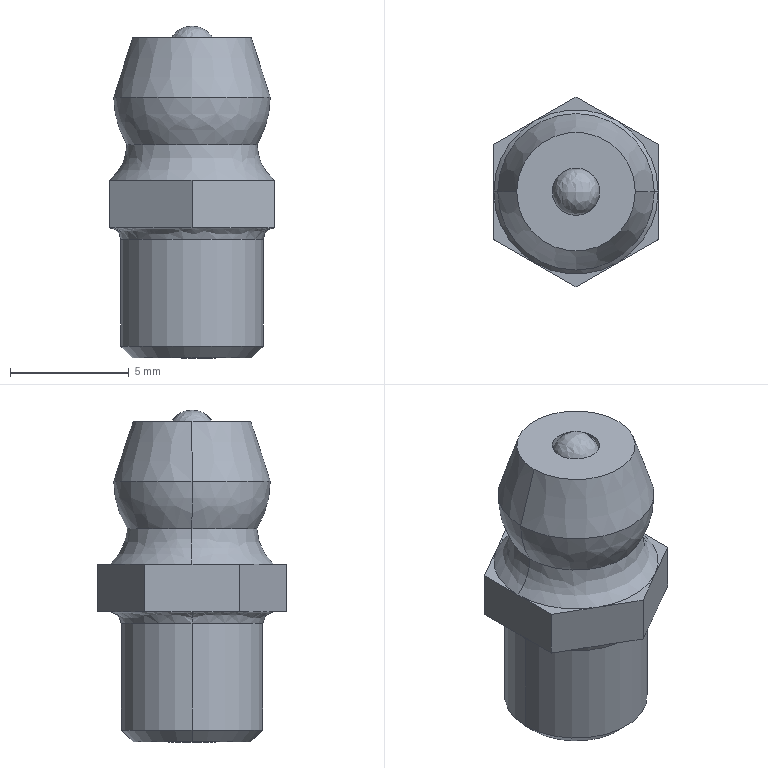Part | STEP file | M6 grease nipple^FTH120-PD-direct-drive motor | 2 solids | 36 faces | box 6.928 x 8 x 13.96 mm | volume 368.725 mm3 | plane 20 | spline 8 | cylinder 4 | cone 4 | commonest cylinder face diameters 2 x2 6 x2
STEP:
#1=CARTESIAN_POINT('',(-1.,0.,13.));
#2=VERTEX_POINT('',#1);
#3=CARTESIAN_POINT('',(1.,0.,13.));
#4=VERTEX_POINT('',#3);
#5=CARTESIAN_POINT('',(0.,0.,13.));
#6=DIRECTION('',(0.,0.,-1.));
#7=DIRECTION('',(-1.,0.,0.));
#8=AXIS2_PLACEMENT_3D('',#5,#6,#7);
#9=CIRCLE('',#8,1.);
#10=EDGE_CURVE('',#2,#4,#9,.T.);
#11=ORIENTED_EDGE('',*,*,#10,.F.);
#12=CARTESIAN_POINT('',(0.,0.,13.));
#13=DIRECTION('',(0.,0.,1.));
#14=DIRECTION('',(-1.,0.,0.));
#15=AXIS2_PLACEMENT_3D('',#12,#13,#14);
#16=CIRCLE('',#15,1.);
#17=EDGE_CURVE('',#2,#4,#16,.T.);
#18=ORIENTED_EDGE('',*,*,#17,.T.);
#19=EDGE_LOOP('',(#11,#18));
#20=FACE_OUTER_BOUND('',#19,.T.);
#21=CARTESIAN_POINT('',(-1.,0.,13.));
#22=CARTESIAN_POINT('',(-1.,0.,13.));
#23=CARTESIAN_POINT('',(-1.,0.,13.));
#24=CARTESIAN_POINT('',(-1.,0.,13.));
#25=CARTESIAN_POINT('',(-1.,-2.,13.));
#26=CARTESIAN_POINT('',(-1.,-2.,17.));
#27=CARTESIAN_POINT('',(-1.,2.,17.));
#28=CARTESIAN_POINT('',(-1.,2.,13.));
#29=CARTESIAN_POINT('',(1.,-2.,13.));
#30=CARTESIAN_POINT('',(1.,-2.,17.));
#31=CARTESIAN_POINT('',(1.,2.,17.));
#32=CARTESIAN_POINT('',(1.,2.,13.));
#33=CARTESIAN_POINT('',(1.,0.,13.));
#34=CARTESIAN_POINT('',(1.,0.,13.));
#35=CARTESIAN_POINT('',(1.,0.,13.));
#36=CARTESIAN_POINT('',(1.,0.,13.));
#37=(BOUNDED_SURFACE()B_SPLINE_SURFACE(3,3,((#21,#22,#23,#24),(#25,#26,#27,#28),(#29,#30,#31,#32),(#33,#34,#35,#36)),.UNSPECIFIED.,.F.,.F.,.T.)B_SPLINE_SURFACE_WITH_KNOTS((4,4),(4,4),(0.,1.),(0.,1.),.UNSPECIFIED.)GEOMETRIC_REPRESENTATION_ITEM()RATIONAL_B_SPLINE_SURFACE(((1.,0.3333,0.3333,1.),(0.3333,0.1111,0.1111,0.3333),(0.3333,0.1111,0.1111,0.3333),(1.,0.3333,0.3333,1.)))REPRESENTATION_ITEM('')SURFACE());
#38=ADVANCED_FACE('',(#20),#37,.T.);
#39=ORIENTED_EDGE('',*,*,#17,.F.);
#40=ORIENTED_EDGE('',*,*,#10,.T.);
#41=EDGE_LOOP('',(#39,#40));
#42=FACE_OUTER_BOUND('',#41,.T.);
#43=CARTESIAN_POINT('',(-1.,0.,13.));
#44=CARTESIAN_POINT('',(-1.,0.,13.));
#45=CARTESIAN_POINT('',(-1.,0.,13.));
#46=CARTESIAN_POINT('',(-1.,0.,13.));
#47=CARTESIAN_POINT('',(-1.,2.,13.));
#48=CARTESIAN_POINT('',(-1.,2.,9.));
#49=CARTESIAN_POINT('',(-1.,-2.,9.));
#50=CARTESIAN_POINT('',(-1.,-2.,13.));
#51=CARTESIAN_POINT('',(1.,2.,13.));
#52=CARTESIAN_POINT('',(1.,2.,9.));
#53=CARTESIAN_POINT('',(1.,-2.,9.));
#54=CARTESIAN_POINT('',(1.,-2.,13.));
#55=CARTESIAN_POINT('',(1.,0.,13.));
#56=CARTESIAN_POINT('',(1.,0.,13.));
#57=CARTESIAN_POINT('',(1.,0.,13.));
#58=CARTESIAN_POINT('',(1.,0.,13.));
#59=(BOUNDED_SURFACE()B_SPLINE_SURFACE(3,3,((#43,#44,#45,#46),(#47,#48,#49,#50),(#51,#52,#53,#54),(#55,#56,#57,#58)),.UNSPECIFIED.,.F.,.F.,.T.)B_SPLINE_SURFACE_WITH_KNOTS((4,4),(4,4),(0.,1.),(0.,1.),.UNSPECIFIED.)GEOMETRIC_REPRESENTATION_ITEM()RATIONAL_B_SPLINE_SURFACE(((1.,0.3333,0.3333,1.),(0.3333,0.1111,0.1111,0.3333),(0.3333,0.1111,0.1111,0.3333),(1.,0.3333,0.3333,1.)))REPRESENTATION_ITEM('')SURFACE());
#60=ADVANCED_FACE('',(#42),#59,.T.);
#61=CLOSED_SHELL('',(#38,#60));
#62=MANIFOLD_SOLID_BREP('',#61);
#63=CARTESIAN_POINT('',(3.464,0.,5.499));
#64=VERTEX_POINT('',#63);
#65=CARTESIAN_POINT('',(3.464,0.5,5.5));
#66=VERTEX_POINT('',#65);
#67=CARTESIAN_POINT('',(3.464,0.,5.499));
#68=CARTESIAN_POINT('',(3.464,0.1667,5.499));
#69=CARTESIAN_POINT('',(3.464,0.3333,5.5));
#70=CARTESIAN_POINT('',(3.464,0.5,5.5));
#71=B_SPLINE_CURVE_WITH_KNOTS('',3,(#67,#68,#69,#70),.UNSPECIFIED.,.F.,.F.,(4,4),(0.,0.0005),.UNSPECIFIED.);
#72=EDGE_CURVE('',#64,#66,#71,.T.);
#73=ORIENTED_EDGE('',*,*,#72,.F.);
#74=CARTESIAN_POINT('',(3.,0.,5.));
#75=VERTEX_POINT('',#74);
#76=CARTESIAN_POINT('',(3.5,0.,5.));
#77=DIRECTION('',(0.,-1.,0.));
#78=DIRECTION('',(1.,0.,0.));
#79=AXIS2_PLACEMENT_3D('',#76,#77,#78);
#80=CIRCLE('',#79,0.5);
#81=EDGE_CURVE('',#64,#75,#80,.T.);
#82=ORIENTED_EDGE('',*,*,#81,.T.);
#83=CARTESIAN_POINT('',(-3.,0.,5.));
#84=VERTEX_POINT('',#83);
#85=CARTESIAN_POINT('',(0.,0.,5.));
#86=DIRECTION('',(0.,0.,-1.));
#87=DIRECTION('',(-1.,0.,0.));
#88=AXIS2_PLACEMENT_3D('',#85,#86,#87);
#89=CIRCLE('',#88,3.);
#90=EDGE_CURVE('',#84,#75,#89,.T.);
#91=ORIENTED_EDGE('',*,*,#90,.F.);
#92=CARTESIAN_POINT('',(-3.464,0.,5.499));
#93=VERTEX_POINT('',#92);
#94=CARTESIAN_POINT('',(-3.5,0.,5.));
#95=DIRECTION('',(0.,1.,0.));
#96=DIRECTION('',(-1.,0.,0.));
#97=AXIS2_PLACEMENT_3D('',#94,#95,#96);
#98=CIRCLE('',#97,0.5);
#99=EDGE_CURVE('',#93,#84,#98,.T.);
#100=ORIENTED_EDGE('',*,*,#99,.F.);
#101=CARTESIAN_POINT('',(-3.464,0.5,5.5));
#102=VERTEX_POINT('',#101);
#103=CARTESIAN_POINT('',(-3.464,0.5,5.5));
#104=CARTESIAN_POINT('',(-3.464,0.3333,5.5));
#105=CARTESIAN_POINT('',(-3.464,0.1667,5.499));
#106=CARTESIAN_POINT('',(-3.464,0.,5.499));
#107=B_SPLINE_CURVE_WITH_KNOTS('',3,(#103,#104,#105,#106),.UNSPECIFIED.,.F.,.F.,(4,4),(-0.0005,0.),.UNSPECIFIED.);
#108=EDGE_CURVE('',#102,#93,#107,.T.);
#109=ORIENTED_EDGE('',*,*,#108,.F.);
#110=CARTESIAN_POINT('',(-2.165,2.75,5.5));
#111=VERTEX_POINT('',#110);
#112=CARTESIAN_POINT('',(-2.165,2.75,5.5));
#113=CARTESIAN_POINT('',(-2.518,2.472,5.5));
#114=CARTESIAN_POINT('',(-2.807,2.139,5.5));
#115=CARTESIAN_POINT('',(-3.256,1.361,5.5));
#116=CARTESIAN_POINT('',(-3.4,0.9446,5.5));
#117=CARTESIAN_POINT('',(-3.464,0.5,5.5));
#118=B_SPLINE_CURVE_WITH_KNOTS('',3,(#112,#113,#114,#115,#116,#117),.UNSPECIFIED.,.F.,.F.,(4,2,4),(0.,0.5,1.),.UNSPECIFIED.);
#119=EDGE_CURVE('',#111,#102,#118,.T.);
#120=ORIENTED_EDGE('',*,*,#119,.F.);
#121=CARTESIAN_POINT('',(-1.299,3.25,5.5));
#122=VERTEX_POINT('',#121);
#123=CARTESIAN_POINT('',(-1.299,3.25,5.5));
#124=CARTESIAN_POINT('',(-1.443,3.167,5.5));
#125=CARTESIAN_POINT('',(-1.588,3.083,5.499));
#126=CARTESIAN_POINT('',(-1.732,3.,5.499));
#127=CARTESIAN_POINT('',(-1.876,2.917,5.499));
#128=CARTESIAN_POINT('',(-2.021,2.833,5.5));
#129=CARTESIAN_POINT('',(-2.165,2.75,5.5));
#130=B_SPLINE_CURVE_WITH_KNOTS('',3,(#123,#124,#125,#126,#127,#128,#129),.UNSPECIFIED.,.F.,.F.,(4,3,4),(0.,0.0005,0.001),.UNSPECIFIED.);
#131=EDGE_CURVE('',#122,#111,#130,.T.);
#132=ORIENTED_EDGE('',*,*,#131,.F.);
#133=CARTESIAN_POINT('',(1.299,3.25,5.5));
#134=VERTEX_POINT('',#133);
#135=CARTESIAN_POINT('',(1.299,3.25,5.5));
#136=CARTESIAN_POINT('',(0.8822,3.417,5.5));
#137=CARTESIAN_POINT('',(0.4489,3.5,5.5));
#138=CARTESIAN_POINT('',(-0.4489,3.5,5.5));
#139=CARTESIAN_POINT('',(-0.8819,3.417,5.5));
#140=CARTESIAN_POINT('',(-1.299,3.25,5.5));
#141=B_SPLINE_CURVE_WITH_KNOTS('',3,(#135,#136,#137,#138,#139,#140),.UNSPECIFIED.,.F.,.F.,(4,2,4),(0.,0.5,1.),.UNSPECIFIED.);
#142=EDGE_CURVE('',#134,#122,#141,.T.);
#143=ORIENTED_EDGE('',*,*,#142,.F.);
#144=CARTESIAN_POINT('',(2.165,2.75,5.5));
#145=VERTEX_POINT('',#144);
#146=CARTESIAN_POINT('',(2.165,2.75,5.5));
#147=CARTESIAN_POINT('',(2.021,2.833,5.5));
#148=CARTESIAN_POINT('',(1.876,2.917,5.499));
#149=CARTESIAN_POINT('',(1.732,3.,5.499));
#150=CARTESIAN_POINT('',(1.588,3.083,5.499));
#151=CARTESIAN_POINT('',(1.443,3.167,5.5));
#152=CARTESIAN_POINT('',(1.299,3.25,5.5));
#153=B_SPLINE_CURVE_WITH_KNOTS('',3,(#146,#147,#148,#149,#150,#151,#152),.UNSPECIFIED.,.F.,.F.,(4,3,4),(0.,0.0005,0.001),.UNSPECIFIED.);
#154=EDGE_CURVE('',#145,#134,#153,.T.);
#155=ORIENTED_EDGE('',*,*,#154,.F.);
#156=CARTESIAN_POINT('',(3.464,0.5,5.5));
#157=CARTESIAN_POINT('',(3.4,0.9443,5.5));
#158=CARTESIAN_POINT('',(3.255,1.361,5.5));
#159=CARTESIAN_POINT('',(2.807,2.139,5.5));
#160=CARTESIAN_POINT('',(2.518,2.472,5.5));
#161=CARTESIAN_POINT('',(2.165,2.75,5.5));
#162=B_SPLINE_CURVE_WITH_KNOTS('',3,(#156,#157,#158,#159,#160,#161),.UNSPECIFIED.,.F.,.F.,(4,2,4),(0.,0.5,1.),.UNSPECIFIED.);
#163=EDGE_CURVE('',#66,#145,#162,.T.);
#164=ORIENTED_EDGE('',*,*,#163,.F.);
#165=EDGE_LOOP('',(#73,#82,#91,#100,#109,#120,#132,#143,#155,#164));
#166=FACE_OUTER_BOUND('',#165,.T.);
#167=CARTESIAN_POINT('',(-3.5,0.,5.5));
#168=CARTESIAN_POINT('',(-3.5,7.,5.5));
#169=CARTESIAN_POINT('',(3.5,7.,5.5));
#170=CARTESIAN_POINT('',(3.5,0.,5.5));
#171=CARTESIAN_POINT('',(-3.207,0.,5.5));
#172=CARTESIAN_POINT('',(-3.207,6.414,5.5));
#173=CARTESIAN_POINT('',(3.207,6.414,5.5));
#174=CARTESIAN_POINT('',(3.207,0.,5.5));
#175=CARTESIAN_POINT('',(-3.,0.,5.293));
#176=CARTESIAN_POINT('',(-3.,6.,5.293));
#177=CARTESIAN_POINT('',(3.,6.,5.293));
#178=CARTESIAN_POINT('',(3.,0.,5.293));
#179=CARTESIAN_POINT('',(-3.,0.,5.));
#180=CARTESIAN_POINT('',(-3.,6.,5.));
#181=CARTESIAN_POINT('',(3.,6.,5.));
#182=CARTESIAN_POINT('',(3.,0.,5.));
#183=(BOUNDED_SURFACE()B_SPLINE_SURFACE(3,3,((#167,#168,#169,#170),(#171,#172,#173,#174),(#175,#176,#177,#178),(#179,#180,#181,#182)),.UNSPECIFIED.,.F.,.F.,.T.)B_SPLINE_SURFACE_WITH_KNOTS((4,4),(4,4),(0.,1.),(0.,1.),.UNSPECIFIED.)GEOMETRIC_REPRESENTATION_ITEM()RATIONAL_B_SPLINE_SURFACE(((1.,0.3333,0.3333,1.),(0.8047,0.2682,0.2682,0.8047),(0.8047,0.2682,0.2682,0.8047),(1.,0.3333,0.3333,1.)))REPRESENTATION_ITEM('')SURFACE());
#184=ADVANCED_FACE('',(#166),#183,.F.);
#185=CARTESIAN_POINT('',(2.75,0.,9.));
#186=VERTEX_POINT('',#185);
#187=CARTESIAN_POINT('',(-2.75,0.,9.));
#188=VERTEX_POINT('',#187);
#189=CARTESIAN_POINT('',(0.,0.,9.));
#190=DIRECTION('',(0.,0.,1.));
#191=DIRECTION('',(-1.,0.,0.));
#192=AXIS2_PLACEMENT_3D('',#189,#190,#191);
#193=CIRCLE('',#192,2.75);
#194=EDGE_CURVE('',#186,#188,#193,.T.);
#195=ORIENTED_EDGE('',*,*,#194,.F.);
#196=CARTESIAN_POINT('',(3.464,0.,7.5));
#197=VERTEX_POINT('',#196);
#198=CARTESIAN_POINT('',(4.682,0.,9.));
#199=DIRECTION('',(0.,-1.,0.));
#200=DIRECTION('',(1.,0.,0.));
#201=AXIS2_PLACEMENT_3D('',#198,#199,#200);
#202=CIRCLE('',#201,1.932);
#203=EDGE_CURVE('',#186,#197,#202,.T.);
#204=ORIENTED_EDGE('',*,*,#203,.T.);
#205=CARTESIAN_POINT('',(1.732,3.,7.5));
#206=VERTEX_POINT('',#205);
#207=CARTESIAN_POINT('',(0.,0.,7.5));
#208=DIRECTION('',(0.,0.,-1.));
#209=DIRECTION('',(-1.,0.,0.));
#210=AXIS2_PLACEMENT_3D('',#207,#208,#209);
#211=CIRCLE('',#210,3.464);
#212=EDGE_CURVE('',#206,#197,#211,.T.);
#213=ORIENTED_EDGE('',*,*,#212,.F.);
#214=CARTESIAN_POINT('',(-1.732,3.,7.5));
#215=VERTEX_POINT('',#214);
#216=CARTESIAN_POINT('',(0.,0.,7.5));
#217=DIRECTION('',(0.,0.,-1.));
#218=DIRECTION('',(-1.,0.,0.));
#219=AXIS2_PLACEMENT_3D('',#216,#217,#218);
#220=CIRCLE('',#219,3.464);
#221=EDGE_CURVE('',#215,#206,#220,.T.);
#222=ORIENTED_EDGE('',*,*,#221,.F.);
#223=CARTESIAN_POINT('',(-3.464,0.,7.5));
#224=VERTEX_POINT('',#223);
#225=CARTESIAN_POINT('',(0.,0.,7.5));
#226=DIRECTION('',(0.,0.,-1.));
#227=DIRECTION('',(-1.,0.,0.));
#228=AXIS2_PLACEMENT_3D('',#225,#226,#227);
#229=CIRCLE('',#228,3.464);
#230=EDGE_CURVE('',#224,#215,#229,.T.);
#231=ORIENTED_EDGE('',*,*,#230,.F.);
#232=CARTESIAN_POINT('',(-4.682,0.,9.));
#233=DIRECTION('',(0.,1.,0.));
#234=DIRECTION('',(-1.,0.,0.));
#235=AXIS2_PLACEMENT_3D('',#232,#233,#234);
#236=CIRCLE('',#235,1.932);
#237=EDGE_CURVE('',#188,#224,#236,.T.);
#238=ORIENTED_EDGE('',*,*,#237,.F.);
#239=EDGE_LOOP('',(#195,#204,#213,#222,#231,#238));
#240=FACE_OUTER_BOUND('',#239,.T.);
#241=CARTESIAN_POINT('',(-2.75,0.,9.));
#242=CARTESIAN_POINT('',(-2.75,5.5,9.));
#243=CARTESIAN_POINT('',(2.75,5.5,9.));
#244=CARTESIAN_POINT('',(2.75,0.,9.));
#245=CARTESIAN_POINT('',(-2.75,0.,8.408));
#246=CARTESIAN_POINT('',(-2.75,5.5,8.408));
#247=CARTESIAN_POINT('',(2.75,5.5,8.408));
#248=CARTESIAN_POINT('',(2.75,0.,8.408));
#249=CARTESIAN_POINT('',(-3.005,0.,7.873));
#250=CARTESIAN_POINT('',(-3.005,6.009,7.873));
#251=CARTESIAN_POINT('',(3.005,6.009,7.873));
#252=CARTESIAN_POINT('',(3.005,0.,7.873));
#253=CARTESIAN_POINT('',(-3.464,0.,7.5));
#254=CARTESIAN_POINT('',(-3.464,6.928,7.5));
#255=CARTESIAN_POINT('',(3.464,6.928,7.5));
#256=CARTESIAN_POINT('',(3.464,0.,7.5));
#257=(BOUNDED_SURFACE()B_SPLINE_SURFACE(3,3,((#241,#242,#243,#244),(#245,#246,#247,#248),(#249,#250,#251,#252),(#253,#254,#255,#256)),.UNSPECIFIED.,.F.,.F.,.T.)B_SPLINE_SURFACE_WITH_KNOTS((4,4),(4,4),(0.,1.),(0.,1.),.UNSPECIFIED.)GEOMETRIC_REPRESENTATION_ITEM()RATIONAL_B_SPLINE_SURFACE(((1.,0.3333,0.3333,1.),(0.9353,0.3118,0.3118,0.9353),(0.9353,0.3118,0.3118,0.9353),(1.,0.3333,0.3333,1.)))REPRESENTATION_ITEM('')SURFACE());
#258=ADVANCED_FACE('',(#240),#257,.F.);
#259=CARTESIAN_POINT('',(0.,0.,9.));
#260=DIRECTION('',(0.,0.,1.));
#261=DIRECTION('',(-1.,0.,0.));
#262=AXIS2_PLACEMENT_3D('',#259,#260,#261);
#263=CIRCLE('',#262,2.75);
#264=EDGE_CURVE('',#188,#186,#263,.T.);
#265=ORIENTED_EDGE('',*,*,#264,.T.);
#266=CARTESIAN_POINT('',(3.3,0.,11.));
#267=VERTEX_POINT('',#266);
#268=CARTESIAN_POINT('',(-0.6999,0.,11.024));
#269=DIRECTION('',(0.,-1.,0.));
#270=DIRECTION('',(1.,0.,0.));
#271=AXIS2_PLACEMENT_3D('',#268,#269,#270);
#272=CIRCLE('',#271,4.);
#273=EDGE_CURVE('',#186,#267,#272,.T.);
#274=ORIENTED_EDGE('',*,*,#273,.T.);
#275=CARTESIAN_POINT('',(-3.3,0.,11.));
#276=VERTEX_POINT('',#275);
#277=CARTESIAN_POINT('',(0.,0.,11.));
#278=DIRECTION('',(0.,0.,1.));
#279=DIRECTION('',(-1.,0.,0.));
#280=AXIS2_PLACEMENT_3D('',#277,#278,#279);
#281=CIRCLE('',#280,3.3);
#282=EDGE_CURVE('',#276,#267,#281,.T.);
#283=ORIENTED_EDGE('',*,*,#282,.F.);
#284=CARTESIAN_POINT('',(0.6999,0.,11.024));
#285=DIRECTION('',(0.,1.,0.));
#286=DIRECTION('',(-1.,0.,0.));
#287=AXIS2_PLACEMENT_3D('',#284,#285,#286);
#288=CIRCLE('',#287,4.);
#289=EDGE_CURVE('',#188,#276,#288,.T.);
#290=ORIENTED_EDGE('',*,*,#289,.F.);
#291=EDGE_LOOP('',(#265,#274,#283,#290));
#292=FACE_OUTER_BOUND('',#291,.T.);
#293=CARTESIAN_POINT('',(2.75,0.,9.));
#294=CARTESIAN_POINT('',(2.75,-5.5,9.));
#295=CARTESIAN_POINT('',(-2.75,-5.5,9.));
#296=CARTESIAN_POINT('',(-2.75,0.,9.));
#297=CARTESIAN_POINT('',(3.108,0.,9.61));
#298=CARTESIAN_POINT('',(3.108,-6.216,9.61));
#299=CARTESIAN_POINT('',(-3.108,-6.216,9.61));
#300=CARTESIAN_POINT('',(-3.108,0.,9.61));
#301=CARTESIAN_POINT('',(3.296,0.,10.292));
#302=CARTESIAN_POINT('',(3.296,-6.591,10.292));
#303=CARTESIAN_POINT('',(-3.296,-6.591,10.292));
#304=CARTESIAN_POINT('',(-3.296,0.,10.292));
#305=CARTESIAN_POINT('',(3.3,0.,11.));
#306=CARTESIAN_POINT('',(3.3,-6.6,11.));
#307=CARTESIAN_POINT('',(-3.3,-6.6,11.));
#308=CARTESIAN_POINT('',(-3.3,0.,11.));
#309=(BOUNDED_SURFACE()B_SPLINE_SURFACE(3,3,((#293,#294,#295,#296),(#297,#298,#299,#300),(#301,#302,#303,#304),(#305,#306,#307,#308)),.UNSPECIFIED.,.F.,.F.,.T.)B_SPLINE_SURFACE_WITH_KNOTS((4,4),(4,4),(0.,1.),(0.,1.),.UNSPECIFIED.)GEOMETRIC_REPRESENTATION_ITEM()RATIONAL_B_SPLINE_SURFACE(((1.,0.3333,0.3333,1.),(0.9772,0.3257,0.3257,0.9772),(0.9772,0.3257,0.3257,0.9772),(1.,0.3333,0.3333,1.)))REPRESENTATION_ITEM('')SURFACE());
#310=ADVANCED_FACE('',(#292),#309,.T.);
#311=ORIENTED_EDGE('',*,*,#90,.T.);
#312=CARTESIAN_POINT('',(3.,0.,0.5));
#313=VERTEX_POINT('',#312);
#314=CARTESIAN_POINT('',(3.,0.,0.));
#315=DIRECTION('',(0.,0.,-1.));
#316=VECTOR('',#315,1000.);
#317=LINE('',#314,#316);
#318=EDGE_CURVE('',#75,#313,#317,.T.);
#319=ORIENTED_EDGE('',*,*,#318,.T.);
#320=CARTESIAN_POINT('',(-3.,0.,0.5));
#321=VERTEX_POINT('',#320);
#322=CARTESIAN_POINT('',(0.,0.,0.5));
#323=DIRECTION('',(0.,0.,1.));
#324=DIRECTION('',(-1.,0.,0.));
#325=AXIS2_PLACEMENT_3D('',#322,#323,#324);
#326=CIRCLE('',#325,3.);
#327=EDGE_CURVE('',#313,#321,#326,.T.);
#328=ORIENTED_EDGE('',*,*,#327,.T.);
#329=CARTESIAN_POINT('',(-3.,0.,0.));
#330=DIRECTION('',(0.,0.,-1.));
#331=VECTOR('',#330,1000.);
#332=LINE('',#329,#331);
#333=EDGE_CURVE('',#84,#321,#332,.T.);
#334=ORIENTED_EDGE('',*,*,#333,.F.);
#335=EDGE_LOOP('',(#311,#319,#328,#334));
#336=FACE_OUTER_BOUND('',#335,.T.);
#337=CARTESIAN_POINT('',(0.,0.,0.));
#338=DIRECTION('',(0.,0.,-1.));
#339=DIRECTION('',(-1.,0.,0.));
#340=AXIS2_PLACEMENT_3D('',#337,#338,#339);
#341=CYLINDRICAL_SURFACE('',#340,3.);
#342=ADVANCED_FACE('',(#336),#341,.T.);
#343=CARTESIAN_POINT('',(2.5,0.,0.));
#344=VERTEX_POINT('',#343);
#345=CARTESIAN_POINT('',(-2.5,0.,0.));
#346=VERTEX_POINT('',#345);
#347=CARTESIAN_POINT('',(0.,0.,0.));
#348=DIRECTION('',(0.,0.,1.));
#349=DIRECTION('',(1.,0.,0.));
#350=AXIS2_PLACEMENT_3D('',#347,#348,#349);
#351=CIRCLE('',#350,2.5);
#352=EDGE_CURVE('',#344,#346,#351,.T.);
#353=ORIENTED_EDGE('',*,*,#352,.T.);
#354=CARTESIAN_POINT('',(-3.,0.,0.5));
#355=DIRECTION('',(-0.7071,0.,0.7071));
#356=VECTOR('',#355,1000.);
#357=LINE('',#354,#356);
#358=EDGE_CURVE('',#346,#321,#357,.T.);
#359=ORIENTED_EDGE('',*,*,#358,.T.);
#360=ORIENTED_EDGE('',*,*,#327,.F.);
#361=CARTESIAN_POINT('',(3.,0.,0.5));
#362=DIRECTION('',(0.7071,0.,0.7071));
#363=VECTOR('',#362,1000.);
#364=LINE('',#361,#363);
#365=EDGE_CURVE('',#344,#313,#364,.T.);
#366=ORIENTED_EDGE('',*,*,#365,.F.);
#367=EDGE_LOOP('',(#353,#359,#360,#366));
#368=FACE_OUTER_BOUND('',#367,.T.);
#369=CARTESIAN_POINT('',(0.,0.,0.5));
#370=DIRECTION('',(0.,0.,1.));
#371=DIRECTION('',(1.,0.,0.));
#372=AXIS2_PLACEMENT_3D('',#369,#370,#371);
#373=CONICAL_SURFACE('',#372,3.,0.7854);
#374=ADVANCED_FACE('',(#368),#373,.T.);
#375=CARTESIAN_POINT('',(1.,0.,13.5));
#376=VERTEX_POINT('',#375);
#377=CARTESIAN_POINT('',(-1.,0.,13.5));
#378=VERTEX_POINT('',#377);
#379=CARTESIAN_POINT('',(0.,0.,13.5));
#380=DIRECTION('',(0.,0.,-1.));
#381=DIRECTION('',(-1.,0.,0.));
#382=AXIS2_PLACEMENT_3D('',#379,#380,#381);
#383=CIRCLE('',#382,1.);
#384=EDGE_CURVE('',#376,#378,#383,.T.);
#385=ORIENTED_EDGE('',*,*,#384,.F.);
#386=CARTESIAN_POINT('',(1.,0.,0.));
#387=VERTEX_POINT('',#386);
#388=CARTESIAN_POINT('',(1.,0.,13.501));
#389=DIRECTION('',(0.,0.,-1.));
#390=VECTOR('',#389,1000.);
#391=LINE('',#388,#390);
#392=EDGE_CURVE('',#376,#387,#391,.T.);
#393=ORIENTED_EDGE('',*,*,#392,.T.);
#394=CARTESIAN_POINT('',(-1.,0.,0.));
#395=VERTEX_POINT('',#394);
#396=CARTESIAN_POINT('',(0.,0.,0.));
#397=DIRECTION('',(0.,0.,1.));
#398=DIRECTION('',(-1.,0.,0.));
#399=AXIS2_PLACEMENT_3D('',#396,#397,#398);
#400=CIRCLE('',#399,1.);
#401=EDGE_CURVE('',#395,#387,#400,.T.);
#402=ORIENTED_EDGE('',*,*,#401,.F.);
#403=CARTESIAN_POINT('',(-1.,0.,13.501));
#404=DIRECTION('',(0.,0.,-1.));
#405=VECTOR('',#404,1000.);
#406=LINE('',#403,#405);
#407=EDGE_CURVE('',#378,#395,#406,.T.);
#408=ORIENTED_EDGE('',*,*,#407,.F.);
#409=EDGE_LOOP('',(#385,#393,#402,#408));
#410=FACE_OUTER_BOUND('',#409,.T.);
#411=CARTESIAN_POINT('',(0.,0.,13.501));
#412=DIRECTION('',(0.,0.,-1.));
#413=DIRECTION('',(-1.,0.,0.));
#414=AXIS2_PLACEMENT_3D('',#411,#412,#413);
#415=CYLINDRICAL_SURFACE('',#414,1.);
#416=ADVANCED_FACE('',(#410),#415,.F.);
#417=CARTESIAN_POINT('',(2.5,0.,13.5));
#418=VERTEX_POINT('',#417);
#419=CARTESIAN_POINT('',(-2.5,0.,13.5));
#420=VERTEX_POINT('',#419);
#421=CARTESIAN_POINT('',(0.,0.,13.5));
#422=DIRECTION('',(0.,0.,1.));
#423=DIRECTION('',(-1.,0.,0.));
#424=AXIS2_PLACEMENT_3D('',#421,#422,#423);
#425=CIRCLE('',#424,2.5);
#426=EDGE_CURVE('',#418,#420,#425,.T.);
#427=ORIENTED_EDGE('',*,*,#426,.F.);
#428=CARTESIAN_POINT('',(3.3,0.,11.));
#429=DIRECTION('',(0.3048,0.,-0.9524));
#430=VECTOR('',#429,1000.);
#431=LINE('',#428,#430);
#432=EDGE_CURVE('',#418,#267,#431,.T.);
#433=ORIENTED_EDGE('',*,*,#432,.T.);
#434=CARTESIAN_POINT('',(0.,0.,11.));
#435=DIRECTION('',(0.,0.,1.));
#436=DIRECTION('',(-1.,0.,0.));
#437=AXIS2_PLACEMENT_3D('',#434,#435,#436);
#438=CIRCLE('',#437,3.3);
#439=EDGE_CURVE('',#267,#276,#438,.T.);
#440=ORIENTED_EDGE('',*,*,#439,.T.);
#441=CARTESIAN_POINT('',(-3.3,0.,11.));
#442=DIRECTION('',(-0.3048,0.,-0.9524));
#443=VECTOR('',#442,1000.);
#444=LINE('',#441,#443);
#445=EDGE_CURVE('',#420,#276,#444,.T.);
#446=ORIENTED_EDGE('',*,*,#445,.F.);
#447=EDGE_LOOP('',(#427,#433,#440,#446));
#448=FACE_OUTER_BOUND('',#447,.T.);
#449=CARTESIAN_POINT('',(0.,0.,11.));
#450=DIRECTION('',(0.,0.,-1.));
#451=DIRECTION('',(-1.,0.,0.));
#452=AXIS2_PLACEMENT_3D('',#449,#450,#451);
#453=CONICAL_SURFACE('',#452,3.3,0.3097);
#454=ADVANCED_FACE('',(#448),#453,.T.);
#455=ORIENTED_EDGE('',*,*,#318,.F.);
#456=CARTESIAN_POINT('',(0.,0.,5.));
#457=DIRECTION('',(0.,0.,-1.));
#458=DIRECTION('',(-1.,0.,0.));
#459=AXIS2_PLACEMENT_3D('',#456,#457,#458);
#460=CIRCLE('',#459,3.);
#461=EDGE_CURVE('',#75,#84,#460,.T.);
#462=ORIENTED_EDGE('',*,*,#461,.T.);
#463=ORIENTED_EDGE('',*,*,#333,.T.);
#464=CARTESIAN_POINT('',(0.,0.,0.5));
#465=DIRECTION('',(0.,0.,1.));
#466=DIRECTION('',(-1.,0.,0.));
#467=AXIS2_PLACEMENT_3D('',#464,#465,#466);
#468=CIRCLE('',#467,3.);
#469=EDGE_CURVE('',#321,#313,#468,.T.);
#470=ORIENTED_EDGE('',*,*,#469,.T.);
#471=EDGE_LOOP('',(#455,#462,#463,#470));
#472=FACE_OUTER_BOUND('',#471,.T.);
#473=CARTESIAN_POINT('',(0.,0.,0.));
#474=DIRECTION('',(0.,0.,-1.));
#475=DIRECTION('',(-1.,0.,0.));
#476=AXIS2_PLACEMENT_3D('',#473,#474,#475);
#477=CYLINDRICAL_SURFACE('',#476,3.);
#478=ADVANCED_FACE('',(#472),#477,.T.);
#479=ORIENTED_EDGE('',*,*,#358,.F.);
#480=CARTESIAN_POINT('',(0.,0.,0.));
#481=DIRECTION('',(0.,0.,1.));
#482=DIRECTION('',(1.,0.,0.));
#483=AXIS2_PLACEMENT_3D('',#480,#481,#482);
#484=CIRCLE('',#483,2.5);
#485=EDGE_CURVE('',#346,#344,#484,.T.);
#486=ORIENTED_EDGE('',*,*,#485,.T.);
#487=ORIENTED_EDGE('',*,*,#365,.T.);
#488=ORIENTED_EDGE('',*,*,#469,.F.);
#489=EDGE_LOOP('',(#479,#486,#487,#488));
#490=FACE_OUTER_BOUND('',#489,.T.);
#491=CARTESIAN_POINT('',(0.,0.,0.5));
#492=DIRECTION('',(0.,0.,1.));
#493=DIRECTION('',(1.,0.,0.));
#494=AXIS2_PLACEMENT_3D('',#491,#492,#493);
#495=CONICAL_SURFACE('',#494,3.,0.7854);
#496=ADVANCED_FACE('',(#490),#495,.T.);
#497=ORIENTED_EDGE('',*,*,#81,.F.);
#498=CARTESIAN_POINT('',(3.464,-0.5,5.5));
#499=VERTEX_POINT('',#498);
#500=CARTESIAN_POINT('',(3.464,-0.5,5.5));
#501=CARTESIAN_POINT('',(3.464,-0.3333,5.5));
#502=CARTESIAN_POINT('',(3.464,-0.1667,5.499));
#503=CARTESIAN_POINT('',(3.464,0.,5.499));
#504=B_SPLINE_CURVE_WITH_KNOTS('',3,(#500,#501,#502,#503),.UNSPECIFIED.,.F.,.F.,(4,4),(-0.0005,0.),.UNSPECIFIED.);
#505=EDGE_CURVE('',#499,#64,#504,.T.);
#506=ORIENTED_EDGE('',*,*,#505,.F.);
#507=CARTESIAN_POINT('',(2.165,-2.75,5.5));
#508=VERTEX_POINT('',#507);
#509=CARTESIAN_POINT('',(2.165,-2.75,5.5));
#510=CARTESIAN_POINT('',(2.518,-2.472,5.5));
#511=CARTESIAN_POINT('',(2.807,-2.139,5.5));
#512=CARTESIAN_POINT('',(3.256,-1.361,5.5));
#513=CARTESIAN_POINT('',(3.4,-0.9446,5.5));
#514=CARTESIAN_POINT('',(3.464,-0.5,5.5));
#515=B_SPLINE_CURVE_WITH_KNOTS('',3,(#509,#510,#511,#512,#513,#514),.UNSPECIFIED.,.F.,.F.,(4,2,4),(0.,0.5,1.),.UNSPECIFIED.);
#516=EDGE_CURVE('',#508,#499,#515,.T.);
#517=ORIENTED_EDGE('',*,*,#516,.F.);
#518=CARTESIAN_POINT('',(1.299,-3.25,5.5));
#519=VERTEX_POINT('',#518);
#520=CARTESIAN_POINT('',(1.299,-3.25,5.5));
#521=CARTESIAN_POINT('',(1.443,-3.167,5.5));
#522=CARTESIAN_POINT('',(1.588,-3.083,5.499));
#523=CARTESIAN_POINT('',(1.732,-3.,5.499));
#524=CARTESIAN_POINT('',(1.876,-2.917,5.499));
#525=CARTESIAN_POINT('',(2.021,-2.833,5.5));
#526=CARTESIAN_POINT('',(2.165,-2.75,5.5));
#527=B_SPLINE_CURVE_WITH_KNOTS('',3,(#520,#521,#522,#523,#524,#525,#526),.UNSPECIFIED.,.F.,.F.,(4,3,4),(0.,0.0005,0.001),.UNSPECIFIED.);
#528=EDGE_CURVE('',#519,#508,#527,.T.);
#529=ORIENTED_EDGE('',*,*,#528,.F.);
#530=CARTESIAN_POINT('',(-1.299,-3.25,5.5));
#531=VERTEX_POINT('',#530);
#532=CARTESIAN_POINT('',(-1.299,-3.25,5.5));
#533=CARTESIAN_POINT('',(-0.8822,-3.417,5.5));
#534=CARTESIAN_POINT('',(-0.4489,-3.5,5.5));
#535=CARTESIAN_POINT('',(0.4489,-3.5,5.5));
#536=CARTESIAN_POINT('',(0.8819,-3.417,5.5));
#537=CARTESIAN_POINT('',(1.299,-3.25,5.5));
#538=B_SPLINE_CURVE_WITH_KNOTS('',3,(#532,#533,#534,#535,#536,#537),.UNSPECIFIED.,.F.,.F.,(4,2,4),(0.,0.5,1.),.UNSPECIFIED.);
#539=EDGE_CURVE('',#531,#519,#538,.T.);
#540=ORIENTED_EDGE('',*,*,#539,.F.);
#541=CARTESIAN_POINT('',(-2.165,-2.75,5.5));
#542=VERTEX_POINT('',#541);
#543=CARTESIAN_POINT('',(-2.165,-2.75,5.5));
#544=CARTESIAN_POINT('',(-2.021,-2.833,5.5));
#545=CARTESIAN_POINT('',(-1.876,-2.917,5.499));
#546=CARTESIAN_POINT('',(-1.732,-3.,5.499));
#547=CARTESIAN_POINT('',(-1.588,-3.083,5.499));
#548=CARTESIAN_POINT('',(-1.443,-3.167,5.5));
#549=CARTESIAN_POINT('',(-1.299,-3.25,5.5));
#550=B_SPLINE_CURVE_WITH_KNOTS('',3,(#543,#544,#545,#546,#547,#548,#549),.UNSPECIFIED.,.F.,.F.,(4,3,4),(0.,0.0005,0.001),.UNSPECIFIED.);
#551=EDGE_CURVE('',#542,#531,#550,.T.);
#552=ORIENTED_EDGE('',*,*,#551,.F.);
#553=CARTESIAN_POINT('',(-3.464,-0.5,5.5));
#554=VERTEX_POINT('',#553);
#555=CARTESIAN_POINT('',(-3.464,-0.5,5.5));
#556=CARTESIAN_POINT('',(-3.4,-0.9443,5.5));
#557=CARTESIAN_POINT('',(-3.255,-1.361,5.5));
#558=CARTESIAN_POINT('',(-2.807,-2.139,5.5));
#559=CARTESIAN_POINT('',(-2.518,-2.472,5.5));
#560=CARTESIAN_POINT('',(-2.165,-2.75,5.5));
#561=B_SPLINE_CURVE_WITH_KNOTS('',3,(#555,#556,#557,#558,#559,#560),.UNSPECIFIED.,.F.,.F.,(4,2,4),(0.,0.5,1.),.UNSPECIFIED.);
#562=EDGE_CURVE('',#554,#542,#561,.T.);
#563=ORIENTED_EDGE('',*,*,#562,.F.);
#564=CARTESIAN_POINT('',(-3.464,0.,5.499));
#565=CARTESIAN_POINT('',(-3.464,-0.1667,5.499));
#566=CARTESIAN_POINT('',(-3.464,-0.3333,5.5));
#567=CARTESIAN_POINT('',(-3.464,-0.5,5.5));
#568=B_SPLINE_CURVE_WITH_KNOTS('',3,(#564,#565,#566,#567),.UNSPECIFIED.,.F.,.F.,(4,4),(0.,0.0005),.UNSPECIFIED.);
#569=EDGE_CURVE('',#93,#554,#568,.T.);
#570=ORIENTED_EDGE('',*,*,#569,.F.);
#571=ORIENTED_EDGE('',*,*,#99,.T.);
#572=ORIENTED_EDGE('',*,*,#461,.F.);
#573=EDGE_LOOP('',(#497,#506,#517,#529,#540,#552,#563,#570,#571,#572));
#574=FACE_OUTER_BOUND('',#573,.T.);
#575=CARTESIAN_POINT('',(3.5,0.,5.5));
#576=CARTESIAN_POINT('',(3.5,-7.,5.5));
#577=CARTESIAN_POINT('',(-3.5,-7.,5.5));
#578=CARTESIAN_POINT('',(-3.5,0.,5.5));
#579=CARTESIAN_POINT('',(3.207,0.,5.5));
#580=CARTESIAN_POINT('',(3.207,-6.414,5.5));
#581=CARTESIAN_POINT('',(-3.207,-6.414,5.5));
#582=CARTESIAN_POINT('',(-3.207,0.,5.5));
#583=CARTESIAN_POINT('',(3.,0.,5.293));
#584=CARTESIAN_POINT('',(3.,-6.,5.293));
#585=CARTESIAN_POINT('',(-3.,-6.,5.293));
#586=CARTESIAN_POINT('',(-3.,0.,5.293));
#587=CARTESIAN_POINT('',(3.,0.,5.));
#588=CARTESIAN_POINT('',(3.,-6.,5.));
#589=CARTESIAN_POINT('',(-3.,-6.,5.));
#590=CARTESIAN_POINT('',(-3.,0.,5.));
#591=(BOUNDED_SURFACE()B_SPLINE_SURFACE(3,3,((#575,#576,#577,#578),(#579,#580,#581,#582),(#583,#584,#585,#586),(#587,#588,#589,#590)),.UNSPECIFIED.,.F.,.F.,.T.)B_SPLINE_SURFACE_WITH_KNOTS((4,4),(4,4),(0.,1.),(0.,1.),.UNSPECIFIED.)GEOMETRIC_REPRESENTATION_ITEM()RATIONAL_B_SPLINE_SURFACE(((1.,0.3333,0.3333,1.),(0.8047,0.2682,0.2682,0.8047),(0.8047,0.2682,0.2682,0.8047),(1.,0.3333,0.3333,1.)))REPRESENTATION_ITEM('')SURFACE());
#592=ADVANCED_FACE('',(#574),#591,.F.);
#593=ORIENTED_EDGE('',*,*,#401,.T.);
#594=CARTESIAN_POINT('',(0.,0.,0.));
#595=DIRECTION('',(0.,0.,1.));
#596=DIRECTION('',(-1.,0.,0.));
#597=AXIS2_PLACEMENT_3D('',#594,#595,#596);
#598=CIRCLE('',#597,1.);
#599=EDGE_CURVE('',#387,#395,#598,.T.);
#600=ORIENTED_EDGE('',*,*,#599,.T.);
#601=EDGE_LOOP('',(#593,#600));
#602=FACE_BOUND('',#601,.T.);
#603=ORIENTED_EDGE('',*,*,#352,.F.);
#604=ORIENTED_EDGE('',*,*,#485,.F.);
#605=EDGE_LOOP('',(#603,#604));
#606=FACE_OUTER_BOUND('',#605,.T.);
#607=CARTESIAN_POINT('',(0.,0.,0.));
#608=DIRECTION('',(0.,0.,-1.));
#609=DIRECTION('',(-1.,0.,0.));
#610=AXIS2_PLACEMENT_3D('',#607,#608,#609);
#611=PLANE('',#610);
#612=ADVANCED_FACE('',(#602,#606),#611,.T.);
#613=ORIENTED_EDGE('',*,*,#516,.T.);
#614=CARTESIAN_POINT('',(3.464,-2.,5.5));
#615=VERTEX_POINT('',#614);
#616=CARTESIAN_POINT('',(3.464,3.,5.5));
#617=DIRECTION('',(0.,-1.,0.));
#618=VECTOR('',#617,1000.);
#619=LINE('',#616,#618);
#620=EDGE_CURVE('',#499,#615,#619,.T.);
#621=ORIENTED_EDGE('',*,*,#620,.T.);
#622=CARTESIAN_POINT('',(1.732,-3.,5.5));
#623=DIRECTION('',(0.866,0.5,0.));
#624=VECTOR('',#623,1000.);
#625=LINE('',#622,#624);
#626=EDGE_CURVE('',#508,#615,#625,.T.);
#627=ORIENTED_EDGE('',*,*,#626,.F.);
#628=EDGE_LOOP('',(#613,#621,#627));
#629=FACE_OUTER_BOUND('',#628,.T.);
#630=CARTESIAN_POINT('',(0.,3.,5.5));
#631=DIRECTION('',(0.,0.,-1.));
#632=DIRECTION('',(-1.,0.,0.));
#633=AXIS2_PLACEMENT_3D('',#630,#631,#632);
#634=PLANE('',#633);
#635=ADVANCED_FACE('',(#629),#634,.T.);
#636=ORIENTED_EDGE('',*,*,#539,.T.);
#637=CARTESIAN_POINT('',(0.,-4.,5.5));
#638=VERTEX_POINT('',#637);
#639=CARTESIAN_POINT('',(1.732,-3.,5.5));
#640=DIRECTION('',(0.866,0.5,0.));
#641=VECTOR('',#640,1000.);
#642=LINE('',#639,#641);
#643=EDGE_CURVE('',#638,#519,#642,.T.);
#644=ORIENTED_EDGE('',*,*,#643,.F.);
#645=CARTESIAN_POINT('',(-1.732,-3.,5.5));
#646=DIRECTION('',(0.866,-0.5,0.));
#647=VECTOR('',#646,1000.);
#648=LINE('',#645,#647);
#649=EDGE_CURVE('',#531,#638,#648,.T.);
#650=ORIENTED_EDGE('',*,*,#649,.F.);
#651=EDGE_LOOP('',(#636,#644,#650));
#652=FACE_OUTER_BOUND('',#651,.T.);
#653=CARTESIAN_POINT('',(0.,3.,5.5));
#654=DIRECTION('',(0.,0.,-1.));
#655=DIRECTION('',(-1.,0.,0.));
#656=AXIS2_PLACEMENT_3D('',#653,#654,#655);
#657=PLANE('',#656);
#658=ADVANCED_FACE('',(#652),#657,.T.);
#659=ORIENTED_EDGE('',*,*,#562,.T.);
#660=CARTESIAN_POINT('',(-3.464,-2.,5.5));
#661=VERTEX_POINT('',#660);
#662=CARTESIAN_POINT('',(-1.732,-3.,5.5));
#663=DIRECTION('',(0.866,-0.5,0.));
#664=VECTOR('',#663,1000.);
#665=LINE('',#662,#664);
#666=EDGE_CURVE('',#661,#542,#665,.T.);
#667=ORIENTED_EDGE('',*,*,#666,.F.);
#668=CARTESIAN_POINT('',(-3.464,0.,5.5));
#669=DIRECTION('',(0.,-1.,0.));
#670=VECTOR('',#669,1000.);
#671=LINE('',#668,#670);
#672=EDGE_CURVE('',#554,#661,#671,.T.);
#673=ORIENTED_EDGE('',*,*,#672,.F.);
#674=EDGE_LOOP('',(#659,#667,#673));
#675=FACE_OUTER_BOUND('',#674,.T.);
#676=CARTESIAN_POINT('',(0.,3.,5.5));
#677=DIRECTION('',(0.,0.,-1.));
#678=DIRECTION('',(-1.,0.,0.));
#679=AXIS2_PLACEMENT_3D('',#676,#677,#678);
#680=PLANE('',#679);
#681=ADVANCED_FACE('',(#675),#680,.T.);
#682=ORIENTED_EDGE('',*,*,#392,.F.);
#683=CARTESIAN_POINT('',(0.,0.,13.5));
#684=DIRECTION('',(0.,0.,-1.));
#685=DIRECTION('',(-1.,0.,0.));
#686=AXIS2_PLACEMENT_3D('',#683,#684,#685);
#687=CIRCLE('',#686,1.);
#688=EDGE_CURVE('',#378,#376,#687,.T.);
#689=ORIENTED_EDGE('',*,*,#688,.F.);
#690=ORIENTED_EDGE('',*,*,#407,.T.);
#691=ORIENTED_EDGE('',*,*,#599,.F.);
#692=EDGE_LOOP('',(#682,#689,#690,#691));
#693=FACE_OUTER_BOUND('',#692,.T.);
#694=CARTESIAN_POINT('',(0.,0.,13.501));
#695=DIRECTION('',(0.,0.,-1.));
#696=DIRECTION('',(-1.,0.,0.));
#697=AXIS2_PLACEMENT_3D('',#694,#695,#696);
#698=CYLINDRICAL_SURFACE('',#697,1.);
#699=ADVANCED_FACE('',(#693),#698,.F.);
#700=ORIENTED_EDGE('',*,*,#119,.T.);
#701=CARTESIAN_POINT('',(-3.464,2.,5.5));
#702=VERTEX_POINT('',#701);
#703=CARTESIAN_POINT('',(-3.464,0.,5.5));
#704=DIRECTION('',(0.,-1.,0.));
#705=VECTOR('',#704,1000.);
#706=LINE('',#703,#705);
#707=EDGE_CURVE('',#702,#102,#706,.T.);
#708=ORIENTED_EDGE('',*,*,#707,.F.);
#709=CARTESIAN_POINT('',(-1.732,3.,5.5));
#710=DIRECTION('',(-0.866,-0.5,0.));
#711=VECTOR('',#710,1000.);
#712=LINE('',#709,#711);
#713=EDGE_CURVE('',#111,#702,#712,.T.);
#714=ORIENTED_EDGE('',*,*,#713,.F.);
#715=EDGE_LOOP('',(#700,#708,#714));
#716=FACE_OUTER_BOUND('',#715,.T.);
#717=CARTESIAN_POINT('',(0.,3.,5.5));
#718=DIRECTION('',(0.,0.,-1.));
#719=DIRECTION('',(-1.,0.,0.));
#720=AXIS2_PLACEMENT_3D('',#717,#718,#719);
#721=PLANE('',#720);
#722=ADVANCED_FACE('',(#716),#721,.T.);
#723=ORIENTED_EDGE('',*,*,#142,.T.);
#724=CARTESIAN_POINT('',(0.,4.,5.5));
#725=VERTEX_POINT('',#724);
#726=CARTESIAN_POINT('',(-1.732,3.,5.5));
#727=DIRECTION('',(-0.866,-0.5,0.));
#728=VECTOR('',#727,1000.);
#729=LINE('',#726,#728);
#730=EDGE_CURVE('',#725,#122,#729,.T.);
#731=ORIENTED_EDGE('',*,*,#730,.F.);
#732=CARTESIAN_POINT('',(1.732,3.,5.5));
#733=DIRECTION('',(-0.866,0.5,0.));
#734=VECTOR('',#733,1000.);
#735=LINE('',#732,#734);
#736=EDGE_CURVE('',#134,#725,#735,.T.);
#737=ORIENTED_EDGE('',*,*,#736,.F.);
#738=EDGE_LOOP('',(#723,#731,#737));
#739=FACE_OUTER_BOUND('',#738,.T.);
#740=CARTESIAN_POINT('',(0.,3.,5.5));
#741=DIRECTION('',(0.,0.,-1.));
#742=DIRECTION('',(-1.,0.,0.));
#743=AXIS2_PLACEMENT_3D('',#740,#741,#742);
#744=PLANE('',#743);
#745=ADVANCED_FACE('',(#739),#744,.T.);
#746=ORIENTED_EDGE('',*,*,#163,.T.);
#747=CARTESIAN_POINT('',(3.464,2.,5.5));
#748=VERTEX_POINT('',#747);
#749=CARTESIAN_POINT('',(1.732,3.,5.5));
#750=DIRECTION('',(-0.866,0.5,0.));
#751=VECTOR('',#750,1000.);
#752=LINE('',#749,#751);
#753=EDGE_CURVE('',#748,#145,#752,.T.);
#754=ORIENTED_EDGE('',*,*,#753,.F.);
#755=CARTESIAN_POINT('',(3.464,3.,5.5));
#756=DIRECTION('',(0.,-1.,0.));
#757=VECTOR('',#756,1000.);
#758=LINE('',#755,#757);
#759=EDGE_CURVE('',#748,#66,#758,.T.);
#760=ORIENTED_EDGE('',*,*,#759,.T.);
#761=EDGE_LOOP('',(#746,#754,#760));
#762=FACE_OUTER_BOUND('',#761,.T.);
#763=CARTESIAN_POINT('',(0.,3.,5.5));
#764=DIRECTION('',(0.,0.,-1.));
#765=DIRECTION('',(-1.,0.,0.));
#766=AXIS2_PLACEMENT_3D('',#763,#764,#765);
#767=PLANE('',#766);
#768=ADVANCED_FACE('',(#762),#767,.T.);
#769=CARTESIAN_POINT('',(3.464,-2.,7.5));
#770=VERTEX_POINT('',#769);
#771=CARTESIAN_POINT('',(3.464,0.,7.5));
#772=DIRECTION('',(0.,-1.,0.));
#773=VECTOR('',#772,1000.);
#774=LINE('',#771,#773);
#775=EDGE_CURVE('',#197,#770,#774,.T.);
#776=ORIENTED_EDGE('',*,*,#775,.T.);
#777=CARTESIAN_POINT('',(3.464,-2.,-0.001));
#778=DIRECTION('',(0.,0.,-1.));
#779=VECTOR('',#778,1000.);
#780=LINE('',#777,#779);
#781=EDGE_CURVE('',#770,#615,#780,.T.);
#782=ORIENTED_EDGE('',*,*,#781,.T.);
#783=ORIENTED_EDGE('',*,*,#620,.F.);
#784=ORIENTED_EDGE('',*,*,#505,.T.);
#785=ORIENTED_EDGE('',*,*,#72,.T.);
#786=ORIENTED_EDGE('',*,*,#759,.F.);
#787=CARTESIAN_POINT('',(3.464,2.,7.5));
#788=VERTEX_POINT('',#787);
#789=CARTESIAN_POINT('',(3.464,2.,-0.001));
#790=DIRECTION('',(0.,0.,1.));
#791=VECTOR('',#790,1000.);
#792=LINE('',#789,#791);
#793=EDGE_CURVE('',#748,#788,#792,.T.);
#794=ORIENTED_EDGE('',*,*,#793,.T.);
#795=CARTESIAN_POINT('',(3.464,0.,7.5));
#796=DIRECTION('',(0.,-1.,0.));
#797=VECTOR('',#796,1000.);
#798=LINE('',#795,#797);
#799=EDGE_CURVE('',#788,#197,#798,.T.);
#800=ORIENTED_EDGE('',*,*,#799,.T.);
#801=EDGE_LOOP('',(#776,#782,#783,#784,#785,#786,#794,#800));
#802=FACE_OUTER_BOUND('',#801,.T.);
#803=CARTESIAN_POINT('',(3.464,0.,-0.001));
#804=DIRECTION('',(1.,0.,0.));
#805=DIRECTION('',(0.,1.,0.));
#806=AXIS2_PLACEMENT_3D('',#803,#804,#805);
#807=PLANE('',#806);
#808=ADVANCED_FACE('',(#802),#807,.T.);
#809=CARTESIAN_POINT('',(0.,0.,13.5));
#810=DIRECTION('',(0.,0.,1.));
#811=DIRECTION('',(-1.,0.,0.));
#812=AXIS2_PLACEMENT_3D('',#809,#810,#811);
#813=CIRCLE('',#812,2.5);
#814=EDGE_CURVE('',#420,#418,#813,.T.);
#815=ORIENTED_EDGE('',*,*,#814,.T.);
#816=ORIENTED_EDGE('',*,*,#426,.T.);
#817=EDGE_LOOP('',(#815,#816));
#818=FACE_OUTER_BOUND('',#817,.T.);
#819=ORIENTED_EDGE('',*,*,#688,.T.);
#820=ORIENTED_EDGE('',*,*,#384,.T.);
#821=EDGE_LOOP('',(#819,#820));
#822=FACE_BOUND('',#821,.T.);
#823=CARTESIAN_POINT('',(0.,3.3,13.5));
#824=DIRECTION('',(0.,0.,1.));
#825=DIRECTION('',(1.,0.,0.));
#826=AXIS2_PLACEMENT_3D('',#823,#824,#825);
#827=PLANE('',#826);
#828=ADVANCED_FACE('',(#818,#822),#827,.T.);
#829=CARTESIAN_POINT('',(1.732,-3.,7.5));
#830=VERTEX_POINT('',#829);
#831=CARTESIAN_POINT('',(0.,-4.,7.5));
#832=VERTEX_POINT('',#831);
#833=CARTESIAN_POINT('',(1.732,-3.,7.5));
#834=DIRECTION('',(-0.866,-0.5,0.));
#835=VECTOR('',#834,1000.);
#836=LINE('',#833,#835);
#837=EDGE_CURVE('',#830,#832,#836,.T.);
#838=ORIENTED_EDGE('',*,*,#837,.T.);
#839=CARTESIAN_POINT('',(0.,-4.,-0.001));
#840=DIRECTION('',(0.,0.,-1.));
#841=VECTOR('',#840,1000.);
#842=LINE('',#839,#841);
#843=EDGE_CURVE('',#832,#638,#842,.T.);
#844=ORIENTED_EDGE('',*,*,#843,.T.);
#845=ORIENTED_EDGE('',*,*,#643,.T.);
#846=ORIENTED_EDGE('',*,*,#528,.T.);
#847=ORIENTED_EDGE('',*,*,#626,.T.);
#848=ORIENTED_EDGE('',*,*,#781,.F.);
#849=CARTESIAN_POINT('',(1.732,-3.,7.5));
#850=DIRECTION('',(-0.866,-0.5,0.));
#851=VECTOR('',#850,1000.);
#852=LINE('',#849,#851);
#853=EDGE_CURVE('',#770,#830,#852,.T.);
#854=ORIENTED_EDGE('',*,*,#853,.T.);
#855=EDGE_LOOP('',(#838,#844,#845,#846,#847,#848,#854));
#856=FACE_OUTER_BOUND('',#855,.T.);
#857=CARTESIAN_POINT('',(1.732,-3.,-0.001));
#858=DIRECTION('',(0.5,-0.866,0.));
#859=DIRECTION('',(0.866,0.5,0.));
#860=AXIS2_PLACEMENT_3D('',#857,#858,#859);
#861=PLANE('',#860);
#862=ADVANCED_FACE('',(#856),#861,.T.);
#863=ORIENTED_EDGE('',*,*,#853,.F.);
#864=ORIENTED_EDGE('',*,*,#775,.F.);
#865=CARTESIAN_POINT('',(0.,0.,7.5));
#866=DIRECTION('',(0.,0.,-1.));
#867=DIRECTION('',(-1.,0.,0.));
#868=AXIS2_PLACEMENT_3D('',#865,#866,#867);
#869=CIRCLE('',#868,3.464);
#870=EDGE_CURVE('',#197,#830,#869,.T.);
#871=ORIENTED_EDGE('',*,*,#870,.T.);
#872=EDGE_LOOP('',(#863,#864,#871));
#873=FACE_OUTER_BOUND('',#872,.T.);
#874=CARTESIAN_POINT('',(0.,3.3,7.5));
#875=DIRECTION('',(0.,0.,1.));
#876=DIRECTION('',(1.,0.,0.));
#877=AXIS2_PLACEMENT_3D('',#874,#875,#876);
#878=PLANE('',#877);
#879=ADVANCED_FACE('',(#873),#878,.T.);
#880=ORIENTED_EDGE('',*,*,#799,.F.);
#881=CARTESIAN_POINT('',(3.464,2.,7.5));
#882=DIRECTION('',(-0.866,0.5,0.));
#883=VECTOR('',#882,1000.);
#884=LINE('',#881,#883);
#885=EDGE_CURVE('',#788,#206,#884,.T.);
#886=ORIENTED_EDGE('',*,*,#885,.T.);
#887=ORIENTED_EDGE('',*,*,#212,.T.);
#888=EDGE_LOOP('',(#880,#886,#887));
#889=FACE_OUTER_BOUND('',#888,.T.);
#890=CARTESIAN_POINT('',(0.,3.3,7.5));
#891=DIRECTION('',(0.,0.,1.));
#892=DIRECTION('',(1.,0.,0.));
#893=AXIS2_PLACEMENT_3D('',#890,#891,#892);
#894=PLANE('',#893);
#895=ADVANCED_FACE('',(#889),#894,.T.);
#896=ORIENTED_EDGE('',*,*,#885,.F.);
#897=ORIENTED_EDGE('',*,*,#793,.F.);
#898=ORIENTED_EDGE('',*,*,#753,.T.);
#899=ORIENTED_EDGE('',*,*,#154,.T.);
#900=ORIENTED_EDGE('',*,*,#736,.T.);
#901=CARTESIAN_POINT('',(0.,4.,7.5));
#902=VERTEX_POINT('',#901);
#903=CARTESIAN_POINT('',(0.,4.,-0.001));
#904=DIRECTION('',(0.,0.,1.));
#905=VECTOR('',#904,1000.);
#906=LINE('',#903,#905);
#907=EDGE_CURVE('',#725,#902,#906,.T.);
#908=ORIENTED_EDGE('',*,*,#907,.T.);
#909=CARTESIAN_POINT('',(1.732,3.,7.5));
#910=DIRECTION('',(0.866,-0.5,0.));
#911=VECTOR('',#910,1000.);
#912=LINE('',#909,#911);
#913=EDGE_CURVE('',#902,#206,#912,.T.);
#914=ORIENTED_EDGE('',*,*,#913,.T.);
#915=EDGE_LOOP('',(#896,#897,#898,#899,#900,#908,#914));
#916=FACE_OUTER_BOUND('',#915,.T.);
#917=CARTESIAN_POINT('',(1.732,3.,-0.001));
#918=DIRECTION('',(0.5,0.866,0.));
#919=DIRECTION('',(-0.866,0.5,0.));
#920=AXIS2_PLACEMENT_3D('',#917,#918,#919);
#921=PLANE('',#920);
#922=ADVANCED_FACE('',(#916),#921,.T.);
#923=ORIENTED_EDGE('',*,*,#432,.F.);
#924=ORIENTED_EDGE('',*,*,#814,.F.);
#925=ORIENTED_EDGE('',*,*,#445,.T.);
#926=ORIENTED_EDGE('',*,*,#282,.T.);
#927=EDGE_LOOP('',(#923,#924,#925,#926));
#928=FACE_OUTER_BOUND('',#927,.T.);
#929=CARTESIAN_POINT('',(0.,0.,11.));
#930=DIRECTION('',(0.,0.,-1.));
#931=DIRECTION('',(-1.,0.,0.));
#932=AXIS2_PLACEMENT_3D('',#929,#930,#931);
#933=CONICAL_SURFACE('',#932,3.3,0.3097);
#934=ADVANCED_FACE('',(#928),#933,.T.);
#935=CARTESIAN_POINT('',(-1.732,-3.,7.5));
#936=VERTEX_POINT('',#935);
#937=CARTESIAN_POINT('',(-3.464,-2.,7.5));
#938=VERTEX_POINT('',#937);
#939=CARTESIAN_POINT('',(-1.732,-3.,7.5));
#940=DIRECTION('',(-0.866,0.5,0.));
#941=VECTOR('',#940,1000.);
#942=LINE('',#939,#941);
#943=EDGE_CURVE('',#936,#938,#942,.T.);
#944=ORIENTED_EDGE('',*,*,#943,.T.);
#945=CARTESIAN_POINT('',(-3.464,-2.,-0.001));
#946=DIRECTION('',(0.,0.,-1.));
#947=VECTOR('',#946,1000.);
#948=LINE('',#945,#947);
#949=EDGE_CURVE('',#938,#661,#948,.T.);
#950=ORIENTED_EDGE('',*,*,#949,.T.);
#951=ORIENTED_EDGE('',*,*,#666,.T.);
#952=ORIENTED_EDGE('',*,*,#551,.T.);
#953=ORIENTED_EDGE('',*,*,#649,.T.);
#954=ORIENTED_EDGE('',*,*,#843,.F.);
#955=CARTESIAN_POINT('',(-1.732,-3.,7.5));
#956=DIRECTION('',(-0.866,0.5,0.));
#957=VECTOR('',#956,1000.);
#958=LINE('',#955,#957);
#959=EDGE_CURVE('',#832,#936,#958,.T.);
#960=ORIENTED_EDGE('',*,*,#959,.T.);
#961=EDGE_LOOP('',(#944,#950,#951,#952,#953,#954,#960));
#962=FACE_OUTER_BOUND('',#961,.T.);
#963=CARTESIAN_POINT('',(-1.732,-3.,-0.001));
#964=DIRECTION('',(-0.5,-0.866,0.));
#965=DIRECTION('',(0.866,-0.5,0.));
#966=AXIS2_PLACEMENT_3D('',#963,#964,#965);
#967=PLANE('',#966);
#968=ADVANCED_FACE('',(#962),#967,.T.);
#969=ORIENTED_EDGE('',*,*,#959,.F.);
#970=ORIENTED_EDGE('',*,*,#837,.F.);
#971=CARTESIAN_POINT('',(0.,0.,7.5));
#972=DIRECTION('',(0.,0.,-1.));
#973=DIRECTION('',(-1.,0.,0.));
#974=AXIS2_PLACEMENT_3D('',#971,#972,#973);
#975=CIRCLE('',#974,3.464);
#976=EDGE_CURVE('',#830,#936,#975,.T.);
#977=ORIENTED_EDGE('',*,*,#976,.T.);
#978=EDGE_LOOP('',(#969,#970,#977));
#979=FACE_OUTER_BOUND('',#978,.T.);
#980=CARTESIAN_POINT('',(0.,3.3,7.5));
#981=DIRECTION('',(0.,0.,1.));
#982=DIRECTION('',(1.,0.,0.));
#983=AXIS2_PLACEMENT_3D('',#980,#981,#982);
#984=PLANE('',#983);
#985=ADVANCED_FACE('',(#979),#984,.T.);
#986=ORIENTED_EDGE('',*,*,#203,.F.);
#987=ORIENTED_EDGE('',*,*,#264,.F.);
#988=ORIENTED_EDGE('',*,*,#237,.T.);
#989=CARTESIAN_POINT('',(0.,0.,7.5));
#990=DIRECTION('',(0.,0.,-1.));
#991=DIRECTION('',(-1.,0.,0.));
#992=AXIS2_PLACEMENT_3D('',#989,#990,#991);
#993=CIRCLE('',#992,3.464);
#994=EDGE_CURVE('',#936,#224,#993,.T.);
#995=ORIENTED_EDGE('',*,*,#994,.F.);
#996=ORIENTED_EDGE('',*,*,#976,.F.);
#997=ORIENTED_EDGE('',*,*,#870,.F.);
#998=EDGE_LOOP('',(#986,#987,#988,#995,#996,#997));
#999=FACE_OUTER_BOUND('',#998,.T.);
#1000=CARTESIAN_POINT('',(2.75,0.,9.));
#1001=CARTESIAN_POINT('',(2.75,-5.5,9.));
#1002=CARTESIAN_POINT('',(-2.75,-5.5,9.));
#1003=CARTESIAN_POINT('',(-2.75,0.,9.));
#1004=CARTESIAN_POINT('',(2.75,0.,8.408));
#1005=CARTESIAN_POINT('',(2.75,-5.5,8.408));
#1006=CARTESIAN_POINT('',(-2.75,-5.5,8.408));
#1007=CARTESIAN_POINT('',(-2.75,0.,8.408));
#1008=CARTESIAN_POINT('',(3.005,0.,7.873));
#1009=CARTESIAN_POINT('',(3.005,-6.009,7.873));
#1010=CARTESIAN_POINT('',(-3.005,-6.009,7.873));
#1011=CARTESIAN_POINT('',(-3.005,0.,7.873));
#1012=CARTESIAN_POINT('',(3.464,0.,7.5));
#1013=CARTESIAN_POINT('',(3.464,-6.928,7.5));
#1014=CARTESIAN_POINT('',(-3.464,-6.928,7.5));
#1015=CARTESIAN_POINT('',(-3.464,0.,7.5));
#1016=(BOUNDED_SURFACE()B_SPLINE_SURFACE(3,3,((#1000,#1001,#1002,#1003),(#1004,#1005,#1006,#1007),(#1008,#1009,#1010,#1011),(#1012,#1013,#1014,#1015)),.UNSPECIFIED.,.F.,.F.,.T.)B_SPLINE_SURFACE_WITH_KNOTS((4,4),(4,4),(0.,1.),(0.,1.),.UNSPECIFIED.)GEOMETRIC_REPRESENTATION_ITEM()RATIONAL_B_SPLINE_SURFACE(((1.,0.3333,0.3333,1.),(0.9353,0.3118,0.3118,0.9353),(0.9353,0.3118,0.3118,0.9353),(1.,0.3333,0.3333,1.)))REPRESENTATION_ITEM('')SURFACE());
#1017=ADVANCED_FACE('',(#999),#1016,.F.);
#1018=ORIENTED_EDGE('',*,*,#913,.F.);
#1019=CARTESIAN_POINT('',(0.,4.,7.5));
#1020=DIRECTION('',(-0.866,-0.5,0.));
#1021=VECTOR('',#1020,1000.);
#1022=LINE('',#1019,#1021);
#1023=EDGE_CURVE('',#902,#215,#1022,.T.);
#1024=ORIENTED_EDGE('',*,*,#1023,.T.);
#1025=ORIENTED_EDGE('',*,*,#221,.T.);
#1026=EDGE_LOOP('',(#1018,#1024,#1025));
#1027=FACE_OUTER_BOUND('',#1026,.T.);
#1028=CARTESIAN_POINT('',(0.,3.3,7.5));
#1029=DIRECTION('',(0.,0.,1.));
#1030=DIRECTION('',(1.,0.,0.));
#1031=AXIS2_PLACEMENT_3D('',#1028,#1029,#1030);
#1032=PLANE('',#1031);
#1033=ADVANCED_FACE('',(#1027),#1032,.T.);
#1034=ORIENTED_EDGE('',*,*,#1023,.F.);
#1035=ORIENTED_EDGE('',*,*,#907,.F.);
#1036=ORIENTED_EDGE('',*,*,#730,.T.);
#1037=ORIENTED_EDGE('',*,*,#131,.T.);
#1038=ORIENTED_EDGE('',*,*,#713,.T.);
#1039=CARTESIAN_POINT('',(-3.464,2.,7.5));
#1040=VERTEX_POINT('',#1039);
#1041=CARTESIAN_POINT('',(-3.464,2.,-0.001));
#1042=DIRECTION('',(0.,0.,1.));
#1043=VECTOR('',#1042,1000.);
#1044=LINE('',#1041,#1043);
#1045=EDGE_CURVE('',#702,#1040,#1044,.T.);
#1046=ORIENTED_EDGE('',*,*,#1045,.T.);
#1047=CARTESIAN_POINT('',(-1.732,3.,7.5));
#1048=DIRECTION('',(0.866,0.5,0.));
#1049=VECTOR('',#1048,1000.);
#1050=LINE('',#1047,#1049);
#1051=EDGE_CURVE('',#1040,#215,#1050,.T.);
#1052=ORIENTED_EDGE('',*,*,#1051,.T.);
#1053=EDGE_LOOP('',(#1034,#1035,#1036,#1037,#1038,#1046,#1052));
#1054=FACE_OUTER_BOUND('',#1053,.T.);
#1055=CARTESIAN_POINT('',(-1.732,3.,-0.001));
#1056=DIRECTION('',(-0.5,0.866,0.));
#1057=DIRECTION('',(-0.866,-0.5,0.));
#1058=AXIS2_PLACEMENT_3D('',#1055,#1056,#1057);
#1059=PLANE('',#1058);
#1060=ADVANCED_FACE('',(#1054),#1059,.T.);
#1061=ORIENTED_EDGE('',*,*,#273,.F.);
#1062=ORIENTED_EDGE('',*,*,#194,.T.);
#1063=ORIENTED_EDGE('',*,*,#289,.T.);
#1064=ORIENTED_EDGE('',*,*,#439,.F.);
#1065=EDGE_LOOP('',(#1061,#1062,#1063,#1064));
#1066=FACE_OUTER_BOUND('',#1065,.T.);
#1067=CARTESIAN_POINT('',(-2.75,0.,9.));
#1068=CARTESIAN_POINT('',(-2.75,5.5,9.));
#1069=CARTESIAN_POINT('',(2.75,5.5,9.));
#1070=CARTESIAN_POINT('',(2.75,0.,9.));
#1071=CARTESIAN_POINT('',(-3.108,0.,9.61));
#1072=CARTESIAN_POINT('',(-3.108,6.216,9.61));
#1073=CARTESIAN_POINT('',(3.108,6.216,9.61));
#1074=CARTESIAN_POINT('',(3.108,0.,9.61));
#1075=CARTESIAN_POINT('',(-3.296,0.,10.292));
#1076=CARTESIAN_POINT('',(-3.296,6.591,10.292));
#1077=CARTESIAN_POINT('',(3.296,6.591,10.292));
#1078=CARTESIAN_POINT('',(3.296,0.,10.292));
#1079=CARTESIAN_POINT('',(-3.3,0.,11.));
#1080=CARTESIAN_POINT('',(-3.3,6.6,11.));
#1081=CARTESIAN_POINT('',(3.3,6.6,11.));
#1082=CARTESIAN_POINT('',(3.3,0.,11.));
#1083=(BOUNDED_SURFACE()B_SPLINE_SURFACE(3,3,((#1067,#1068,#1069,#1070),(#1071,#1072,#1073,#1074),(#1075,#1076,#1077,#1078),(#1079,#1080,#1081,#1082)),.UNSPECIFIED.,.F.,.F.,.T.)B_SPLINE_SURFACE_WITH_KNOTS((4,4),(4,4),(0.,1.),(0.,1.),.UNSPECIFIED.)GEOMETRIC_REPRESENTATION_ITEM()RATIONAL_B_SPLINE_SURFACE(((1.,0.3333,0.3333,1.),(0.9772,0.3257,0.3257,0.9772),(0.9772,0.3257,0.3257,0.9772),(1.,0.3333,0.3333,1.)))REPRESENTATION_ITEM('')SURFACE());
#1084=ADVANCED_FACE('',(#1066),#1083,.T.);
#1085=CARTESIAN_POINT('',(-3.464,0.,7.5));
#1086=DIRECTION('',(0.,1.,0.));
#1087=VECTOR('',#1086,1000.);
#1088=LINE('',#1085,#1087);
#1089=EDGE_CURVE('',#224,#1040,#1088,.T.);
#1090=ORIENTED_EDGE('',*,*,#1089,.T.);
#1091=ORIENTED_EDGE('',*,*,#1045,.F.);
#1092=ORIENTED_EDGE('',*,*,#707,.T.);
#1093=ORIENTED_EDGE('',*,*,#108,.T.);
#1094=ORIENTED_EDGE('',*,*,#569,.T.);
#1095=ORIENTED_EDGE('',*,*,#672,.T.);
#1096=ORIENTED_EDGE('',*,*,#949,.F.);
#1097=CARTESIAN_POINT('',(-3.464,0.,7.5));
#1098=DIRECTION('',(0.,1.,0.));
#1099=VECTOR('',#1098,1000.);
#1100=LINE('',#1097,#1099);
#1101=EDGE_CURVE('',#938,#224,#1100,.T.);
#1102=ORIENTED_EDGE('',*,*,#1101,.T.);
#1103=EDGE_LOOP('',(#1090,#1091,#1092,#1093,#1094,#1095,#1096,#1102));
#1104=FACE_OUTER_BOUND('',#1103,.T.);
#1105=CARTESIAN_POINT('',(-3.464,0.,-0.001));
#1106=DIRECTION('',(-1.,0.,0.));
#1107=DIRECTION('',(0.,0.,1.));
#1108=AXIS2_PLACEMENT_3D('',#1105,#1106,#1107);
#1109=PLANE('',#1108);
#1110=ADVANCED_FACE('',(#1104),#1109,.T.);
#1111=ORIENTED_EDGE('',*,*,#1101,.F.);
#1112=ORIENTED_EDGE('',*,*,#943,.F.);
#1113=ORIENTED_EDGE('',*,*,#994,.T.);
#1114=EDGE_LOOP('',(#1111,#1112,#1113));
#1115=FACE_OUTER_BOUND('',#1114,.T.);
#1116=CARTESIAN_POINT('',(0.,3.3,7.5));
#1117=DIRECTION('',(0.,0.,1.));
#1118=DIRECTION('',(1.,0.,0.));
#1119=AXIS2_PLACEMENT_3D('',#1116,#1117,#1118);
#1120=PLANE('',#1119);
#1121=ADVANCED_FACE('',(#1115),#1120,.T.);
#1122=ORIENTED_EDGE('',*,*,#1051,.F.);
#1123=ORIENTED_EDGE('',*,*,#1089,.F.);
#1124=ORIENTED_EDGE('',*,*,#230,.T.);
#1125=EDGE_LOOP('',(#1122,#1123,#1124));
#1126=FACE_OUTER_BOUND('',#1125,.T.);
#1127=CARTESIAN_POINT('',(0.,3.3,7.5));
#1128=DIRECTION('',(0.,0.,1.));
#1129=DIRECTION('',(1.,0.,0.));
#1130=AXIS2_PLACEMENT_3D('',#1127,#1128,#1129);
#1131=PLANE('',#1130);
#1132=ADVANCED_FACE('',(#1126),#1131,.T.);
#1133=CLOSED_SHELL('',(#184,#258,#310,#342,#374,#416,#454,#478,#496,#592,#612,#635,#658,#681,#699,#722,#745,#768,#808,#828,#862,#879,#895,#922,#934,#968,#985,#1017,#1033,#1060,#1084,#1110,#1121,#1132));
#1134=MANIFOLD_SOLID_BREP('',#1133);
#1135=CARTESIAN_POINT('',(0.,0.,0.));
#1136=DIRECTION('',(0.,0.,1.));
#1137=DIRECTION('',(1.,0.,0.));
#1138=AXIS2_PLACEMENT_3D('',#1135,#1136,#1137);
#1139=(LENGTH_UNIT()NAMED_UNIT(*)SI_UNIT(.MILLI.,.METRE.));
#1140=UNCERTAINTY_MEASURE_WITH_UNIT(LENGTH_MEASURE(0.00001),#1139,'','');
#1141=(NAMED_UNIT(*)PLANE_ANGLE_UNIT()SI_UNIT($,.RADIAN.));
#1142=(NAMED_UNIT(*)SI_UNIT($,.STERADIAN.)SOLID_ANGLE_UNIT());
#1143=(GEOMETRIC_REPRESENTATION_CONTEXT(3)GLOBAL_UNCERTAINTY_ASSIGNED_CONTEXT((#1140))GLOBAL_UNIT_ASSIGNED_CONTEXT((#1139,#1141,#1142))REPRESENTATION_CONTEXT('',''));
#1144=ADVANCED_BREP_SHAPE_REPRESENTATION('',(#62,#1134,#1138),#1143);